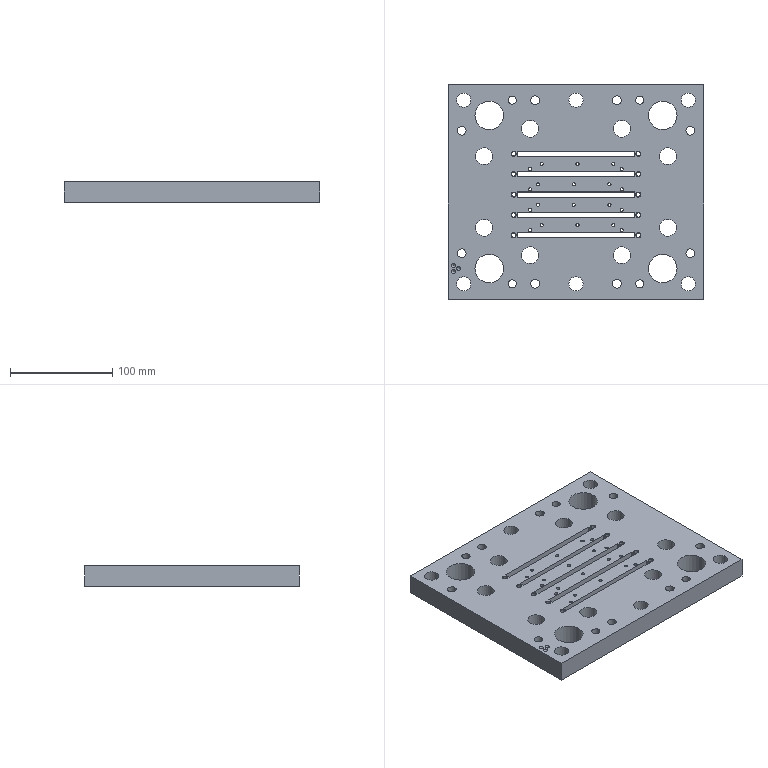Part | STEP file | 200 mesh_id2098 | 1 solid | 125 faces | box 250 x 210 x 20 mm | volume 863809 mm3 | cylinder 68 | plane 34 | cone 23 | commonest cylinder face diameters 3.1 x20 14 x14 4.2 x10 8.6 x8 16.5 x8 8 x4